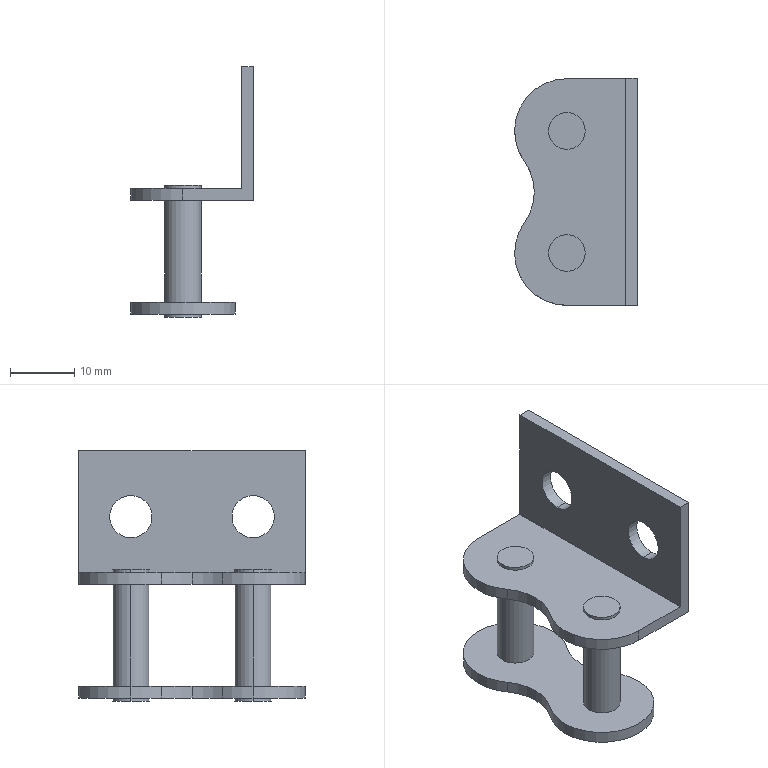Part | STEP file | IN_01_01_07_01_03 | 1 solid | 42 faces | box 19.15 x 35.35 x 39.1 mm | volume 3982 mm3 | cylinder 29 | plane 13 | commonest cylinder face diameters 16.3 x13 5.72 x12 6.6 x4